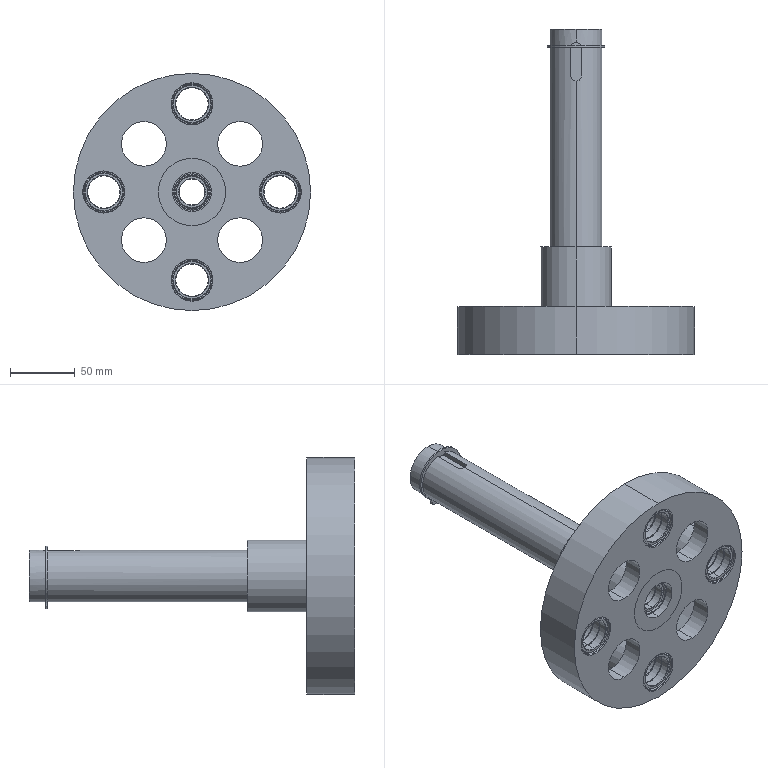Part | SolidWorks | 31 solids | 4701 faces | volume 671683 mm3 | spline 4131 | cylinder 426 | plane 142 | cone 2 | commonest cylinder face diameters 29 x80 33 x80 37 x54 25 x40 20 x22 24 x20